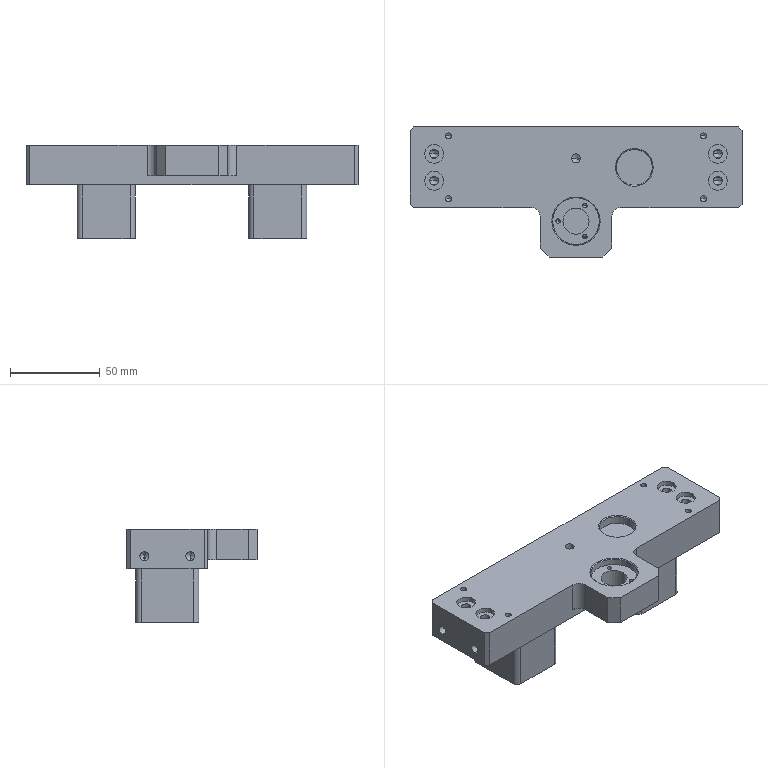NC program | NX | posted with a generic post | part box 185 x 72.5 x 52 mm
Lines 57 to 1270 of 6926:
(CAVITY_MILL , TOOL : D10)
N100 T15 M6
N102 G54
N104 G17 G0 G90 X-4.33 Y48.246 S9500 M3
N106 G43 Z30. H15
N108 Z0.003
N110 G94 G1 Z-0.997 F700.
N112 X-0.866 Y42.246
N114 G3 X0. Y41.746 R1.
N116 G1 X97.503 F2500.
N118 G2 X97.996 Y41.253 R0.493
N120 G1 Y-41.253
N122 G2 X97.503 Y-41.746 R0.493
N124 G1 X-97.503
N126 G2 X-97.996 Y-41.253 R0.493
N128 G1 Y41.253
N130 G2 X-97.503 Y41.746 R0.493
N132 G1 X0.
N134 Y36.746
N136 X92.996
N138 Y-36.746
N140 X64.26
N142 G3 X70.1 Y-28.25 R9.1
N144 G1 Y0.75
N146 G3 X61. Y9.85 R9.1
N148 G1 X34.5
N150 G3 X25.4 Y0.75 R9.1
N152 G1 Y-28.25
N154 G3 X31.24 Y-36.746 R9.1
N156 G1 X31.598 Y-35.812
N158 G2 X26.4 Y-28.25 R8.1
N160 G1 Y0.75
N162 G2 X34.5 Y8.85 R8.1
N164 G1 X61.
N166 G2 X69.1 Y0.75 R8.1
N168 G1 Y-28.25
N170 G2 X61. Y-36.35 R8.1
N172 G1 X34.5
N174 G2 X31.598 Y-35.812 R8.1
N176 G1 X31.24 Y-36.746
N178 X-31.24
N180 G3 X-25.4 Y-28.25 R9.1
N182 G1 Y0.75
N184 G3 X-34.5 Y9.85 R9.1
N186 G1 X-61.
N188 G3 X-70.1 Y0.75 R9.1
N190 G1 Y-28.25
N192 G3 X-64.26 Y-36.746 R9.1
N194 G1 X-63.902 Y-35.812
N196 G2 X-69.1 Y-28.25 R8.1
N198 G1 Y0.75
N200 G2 X-61. Y8.85 R8.1
N202 G1 X-34.5
N204 G2 X-26.4 Y0.75 R8.1
N206 G1 Y-28.25
N208 G2 X-34.5 Y-36.35 R8.1
N210 G1 X-61.
N212 G2 X-63.902 Y-35.812 R8.1
N214 G1 X-64.26 Y-36.746
N216 X-92.996
N218 Y36.746
N220 X0.
N222 Y31.746
N224 X87.996
N226 Y-31.746
N228 X74.66
N230 G3 X75.1 Y-28.25 R14.1
N232 G1 Y0.75
N234 G3 X61. Y14.85 R14.1
N236 G1 X34.5
N238 G3 X20.4 Y0.75 R14.1
N240 G1 Y-28.25
N242 G3 X20.84 Y-31.746 R14.1
N244 G1 X-20.84
N246 G3 X-20.4 Y-28.25 R14.1
N248 G1 Y0.75
N250 G3 X-34.5 Y14.85 R14.1
N252 G1 X-61.
N254 G3 X-75.1 Y0.75 R14.1
N256 G1 Y-28.25
N258 G3 X-74.66 Y-31.746 R14.1
N260 G1 X-87.996
N262 Y31.746
N264 X0.
N266 Y26.746
N268 X82.996
N270 Y-26.746
N272 X80.1
N274 Y0.75
N276 G3 X70.376 Y17.39 R19.1
N278 G1 X72.831 Y21.746
N280 X77.996
N282 Y17.836
N284 G3 X72.831 Y21.746 R24.1
N286 G1 X70.376 Y17.39
N288 G3 X61. Y19.85 R19.1
N290 G1 X34.5
N292 G3 X15.4 Y0.75 R19.1
N294 G1 Y-26.746
N296 X-15.4
N298 Y0.75
N300 G3 X-34.5 Y19.85 R19.1
N302 G1 X-61.
N304 G3 X-80.1 Y0.75 R19.1
N306 G1 Y-26.746
N308 X-82.996
N310 Y26.746
N312 X-72.831
N314 Y21.746
N316 G3 X-77.996 Y17.836 R24.1
N318 G1 Y21.746
N320 X-72.831
N322 Y26.746
N324 X0.
N326 Y21.746
N328 X22.669
N330 G3 X10.4 Y0.75 R24.1
N332 G1 Y-21.746
N334 X-10.4
N336 Y0.75
N338 G3 X-22.669 Y21.746 R24.1
N340 G1 X0.
N342 Y16.746
N344 X10.191
N346 G3 X5.4 Y0.75 R29.1
N348 G1 Y-16.746
N350 X-5.4
N352 Y0.75
N354 G3 X-10.191 Y16.746 R29.1
N356 G1 X0.
N358 Y11.746
N360 X2.222
N362 G3 X0.4 Y0.75 R34.1
N364 G1 Y-11.746
N366 X-0.4
N368 Y0.75
N370 G3 X-2.222 Y11.746 R34.1
N372 G1 X0.
N374 G3 X0.866 Y12.246 R1.
N376 G1 Z0.003
N378 G0 X-4.33 Y48.246 Z-0.993
N380 G1 Z-1.993 F700.
N382 X-0.866 Y42.246
N384 G3 X0. Y41.746 R1.
N386 G1 X97.503 F2500.
N388 G2 X97.996 Y41.253 R0.493
N390 G1 Y-41.253
N392 G2 X97.503 Y-41.746 R0.493
N394 G1 X-97.503
N396 G2 X-97.996 Y-41.253 R0.493
N398 G1 Y41.253
N400 G2 X-97.503 Y41.746 R0.493
N402 G1 X0.
N404 Y36.746
N406 X92.996
N408 Y-36.746
N410 X64.26
N412 G3 X70.1 Y-28.25 R9.1
N414 G1 Y0.75
N416 G3 X61. Y9.85 R9.1
N418 G1 X34.5
N420 G3 X25.4 Y0.75 R9.1
N422 G1 Y-28.25
N424 G3 X31.24 Y-36.746 R9.1
N426 G1 X31.599 Y-35.813
N428 G2 X26.4 Y-28.25 R8.1
N430 G1 Y0.75
N432 G2 X34.5 Y8.85 R8.1
N434 G1 X61.
N436 G2 X69.1 Y0.75 R8.1
N438 G1 Y-28.25
N440 G2 X61. Y-36.35 R8.1
N442 G1 X34.5
N444 G2 X31.599 Y-35.813 R8.1
N446 G1 X31.24 Y-36.746
N448 X-31.24
N450 G3 X-25.4 Y-28.25 R9.1
N452 G1 Y0.75
N454 G3 X-34.5 Y9.85 R9.1
N456 G1 X-61.
N458 G3 X-70.1 Y0.75 R9.1
N460 G1 Y-28.25
N462 G3 X-64.26 Y-36.746 R9.1
N464 G1 X-63.901 Y-35.813
N466 G2 X-69.1 Y-28.25 R8.1
N468 G1 Y0.75
N470 G2 X-61. Y8.85 R8.1
N472 G1 X-34.5
N474 G2 X-26.4 Y0.75 R8.1
N476 G1 Y-28.25
N478 G2 X-34.5 Y-36.35 R8.1
N480 G1 X-61.
N482 G2 X-63.901 Y-35.813 R8.1
N484 G1 X-64.26 Y-36.746
N486 X-92.996
N488 Y36.746
N490 X0.
N492 Y31.746
N494 X87.996
N496 Y-31.746
N498 X74.66
N500 G3 X75.1 Y-28.25 R14.1
N502 G1 Y0.75
N504 G3 X61. Y14.85 R14.1
N506 G1 X34.5
N508 G3 X20.4 Y0.75 R14.1
N510 G1 Y-28.25
N512 G3 X20.84 Y-31.746 R14.1
N514 G1 X-20.84
N516 G3 X-20.4 Y-28.25 R14.1
N518 G1 Y0.75
N520 G3 X-34.5 Y14.85 R14.1
N522 G1 X-61.
N524 G3 X-75.1 Y0.75 R14.1
N526 G1 Y-28.25
N528 G3 X-74.66 Y-31.746 R14.1
N530 G1 X-87.996
N532 Y31.746
N534 X0.
N536 Y26.746
N538 X82.996
N540 Y-26.746
N542 X80.1
N544 Y0.75
N546 G3 X70.376 Y17.39 R19.1
N548 G1 X72.831 Y21.746
N550 X77.996
N552 Y17.836
N554 G3 X72.831 Y21.746 R24.1
N556 G1 X70.376 Y17.39
N558 G3 X61. Y19.85 R19.1
N560 G1 X34.5
N562 G3 X15.4 Y0.75 R19.1
N564 G1 Y-26.746
N566 X-15.4
N568 Y0.75
N570 G3 X-34.5 Y19.85 R19.1
N572 G1 X-61.
N574 G3 X-80.1 Y0.75 R19.1
N576 G1 Y-26.746
N578 X-82.996
N580 Y26.746
N582 X-72.831
N584 Y21.746
N586 G3 X-77.996 Y17.836 R24.1
N588 G1 Y21.746
N590 X-72.831
N592 Y26.746
N594 X0.
N596 Y21.746
N598 X22.669
N600 G3 X10.4 Y0.75 R24.1
N602 G1 Y-21.746
N604 X-10.4
N606 Y0.75
N608 G3 X-22.669 Y21.746 R24.1
N610 G1 X0.
N612 Y16.746
N614 X10.191
N616 G3 X5.4 Y0.75 R29.1
N618 G1 Y-16.746
N620 X-5.4
N622 Y0.75
N624 G3 X-10.191 Y16.746 R29.1
N626 G1 X0.
N628 Y11.746
N630 X2.222
N632 G3 X0.4 Y0.75 R34.1
N634 G1 Y-11.746
N636 X-0.4
N638 Y0.75
N640 G3 X-2.222 Y11.746 R34.1
N642 G1 X0.
N644 G3 X0.866 Y12.246 R1.
N646 G1 Z-0.993
N648 G0 X-4.33 Y48.246 Z-1.99
N650 G1 Z-2.99 F700.
N652 X-0.866 Y42.246
N654 G3 X0. Y41.746 R1.
N656 G1 X97.503 F2500.
N658 G2 X97.997 Y41.253 R0.493
N660 G1 Y-41.253
N662 G2 X97.503 Y-41.746 R0.493
N664 G1 X-97.503
N666 G2 X-97.997 Y-41.253 R0.493
N668 G1 Y41.253
N670 G2 X-97.503 Y41.746 R0.493
N672 G1 X0.
N674 Y36.746
N676 X92.997
N678 Y-36.746
N680 X64.259
N682 G3 X70.1 Y-28.25 R9.1
N684 G1 Y0.75
N686 G3 X61. Y9.85 R9.1
N688 G1 X34.5
N690 G3 X25.4 Y0.75 R9.1
N692 G1 Y-28.25
N694 G3 X31.241 Y-36.746 R9.1
N696 G1 X31.599 Y-35.813
N698 G2 X26.4 Y-28.25 R8.1
N700 G1 Y0.75
N702 G2 X34.5 Y8.85 R8.1
N704 G1 X61.
N706 G2 X69.1 Y0.75 R8.1
N708 G1 Y-28.25
N710 G2 X61. Y-36.35 R8.1
N712 G1 X34.5
N714 G2 X31.599 Y-35.813 R8.1
N716 G1 X31.241 Y-36.746
N718 X-31.241
N720 G3 X-25.4 Y-28.25 R9.1
N722 G1 Y0.75
N724 G3 X-34.5 Y9.85 R9.1
N726 G1 X-61.
N728 G3 X-70.1 Y0.75 R9.1
N730 G1 Y-28.25
N732 G3 X-64.259 Y-36.746 R9.1
N734 G1 X-63.901 Y-35.813
N736 G2 X-69.1 Y-28.25 R8.1
N738 G1 Y0.75
N740 G2 X-61. Y8.85 R8.1
N742 G1 X-34.5
N744 G2 X-26.4 Y0.75 R8.1
N746 G1 Y-28.25
N748 G2 X-34.5 Y-36.35 R8.1
N750 G1 X-61.
N752 G2 X-63.901 Y-35.813 R8.1
N754 G1 X-64.259 Y-36.746
N756 X-92.997
N758 Y36.746
N760 X0.
N762 Y31.746
N764 X87.997
N766 Y-31.746
N768 X74.66
N770 G3 X75.1 Y-28.25 R14.1
N772 G1 Y0.75
N774 G3 X61. Y14.85 R14.1
N776 G1 X34.5
N778 G3 X20.4 Y0.75 R14.1
N780 G1 Y-28.25
N782 G3 X20.84 Y-31.746 R14.1
N784 G1 X-20.84
N786 G3 X-20.4 Y-28.25 R14.1
N788 G1 Y0.75
N790 G3 X-34.5 Y14.85 R14.1
N792 G1 X-61.
N794 G3 X-75.1 Y0.75 R14.1
N796 G1 Y-28.25
N798 G3 X-74.66 Y-31.746 R14.1
N800 G1 X-87.997
N802 Y31.746
N804 X0.
N806 Y26.746
N808 X82.997
N810 Y-26.746
N812 X80.1
N814 Y0.75
N816 G3 X70.376 Y17.39 R19.1
N818 G1 X72.831 Y21.746
N820 X77.997
N822 Y17.836
N824 G3 X72.831 Y21.746 R24.1
N826 G1 X70.376 Y17.39
N828 G3 X61. Y19.85 R19.1
N830 G1 X34.5
N832 G3 X15.4 Y0.75 R19.1
N834 G1 Y-26.746
N836 X-15.4
N838 Y0.75
N840 G3 X-34.5 Y19.85 R19.1
N842 G1 X-61.
N844 G3 X-80.1 Y0.75 R19.1
N846 G1 Y-26.746
N848 X-82.997
N850 Y26.746
N852 X-72.831
N854 Y21.746
N856 G3 X-77.997 Y17.836 R24.1
N858 G1 Y21.746
N860 X-72.831
N862 Y26.746
N864 X0.
N866 Y21.746
N868 X22.669
N870 G3 X10.4 Y0.75 R24.1
N872 G1 Y-21.746
N874 X-10.4
N876 Y0.75
N878 G3 X-22.669 Y21.746 R24.1
N880 G1 X0.
N882 Y16.746
N884 X10.191
N886 G3 X5.4 Y0.75 R29.1
N888 G1 Y-16.746
N890 X-5.4
N892 Y0.75
N894 G3 X-10.191 Y16.746 R29.1
N896 G1 X0.
N898 Y11.746
N900 X2.222
N902 G3 X0.4 Y0.75 R34.1
N904 G1 Y-11.746
N906 X-0.4
N908 Y0.75
N910 G3 X-2.222 Y11.746 R34.1
N912 G1 X0.
N914 G3 X0.866 Y12.246 R1.
N916 G1 Z-1.99
N918 G0 X-4.33 Y48.246 Z-2.987
N920 G1 Z-3.987 F700.
N922 X-0.866 Y42.246
N924 G3 X0. Y41.746 R1.
N926 G1 X97.503 F2500.
N928 G2 X97.997 Y41.253 R0.494
N930 G1 Y-41.253
N932 G2 X97.503 Y-41.746 R0.494
N934 G1 X-97.503
N936 G2 X-97.997 Y-41.253 R0.494
N938 G1 Y41.253
N940 G2 X-97.503 Y41.746 R0.494
N942 G1 X0.
N944 Y36.746
N946 X92.997
N948 Y-36.746
N950 X64.259
N952 G3 X70.1 Y-28.25 R9.1
N954 G1 Y0.75
N956 G3 X61. Y9.85 R9.1
N958 G1 X34.5
N960 G3 X25.4 Y0.75 R9.1
N962 G1 Y-28.25
N964 G3 X31.241 Y-36.746 R9.1
N966 G1 X31.599 Y-35.813
N968 G2 X26.4 Y-28.25 R8.1
N970 G1 Y0.75
N972 G2 X34.5 Y8.85 R8.1
N974 G1 X61.
N976 G2 X69.1 Y0.75 R8.1
N978 G1 Y-28.25
N980 G2 X61. Y-36.35 R8.1
N982 G1 X34.5
N984 G2 X31.599 Y-35.813 R8.1
N986 G1 X31.241 Y-36.746
N988 X-31.241
N990 G3 X-25.4 Y-28.25 R9.1
N992 G1 Y0.75
N994 G3 X-34.5 Y9.85 R9.1
N996 G1 X-61.
N998 G3 X-70.1 Y0.75 R9.1
N1000 G1 Y-28.25
N1002 G3 X-64.259 Y-36.746 R9.1
N1004 G1 X-63.901 Y-35.813
N1006 G2 X-69.1 Y-28.25 R8.1
N1008 G1 Y0.75
N1010 G2 X-61. Y8.85 R8.1
N1012 G1 X-34.5
N1014 G2 X-26.4 Y0.75 R8.1
N1016 G1 Y-28.25
N1018 G2 X-34.5 Y-36.35 R8.1
N1020 G1 X-61.
N1022 G2 X-63.901 Y-35.813 R8.1
N1024 G1 X-64.259 Y-36.746
N1026 X-92.997
N1028 Y36.746
N1030 X0.
N1032 Y31.746
N1034 X87.997
N1036 Y-31.746
N1038 X74.66
N1040 G3 X75.1 Y-28.25 R14.1
N1042 G1 Y0.75
N1044 G3 X61. Y14.85 R14.1
N1046 G1 X34.5
N1048 G3 X20.4 Y0.75 R14.1
N1050 G1 Y-28.25
N1052 G3 X20.84 Y-31.746 R14.1
N1054 G1 X-20.84
N1056 G3 X-20.4 Y-28.25 R14.1
N1058 G1 Y0.75
N1060 G3 X-34.5 Y14.85 R14.1
N1062 G1 X-61.
N1064 G3 X-75.1 Y0.75 R14.1
N1066 G1 Y-28.25
N1068 G3 X-74.66 Y-31.746 R14.1
N1070 G1 X-87.997
N1072 Y31.746
N1074 X0.
N1076 Y26.746
N1078 X82.997
N1080 Y-26.746
N1082 X80.1
N1084 Y0.75
N1086 G3 X70.376 Y17.39 R19.1
N1088 G1 X72.831 Y21.746
N1090 X77.997
N1092 Y17.836
N1094 G3 X72.831 Y21.746 R24.1
N1096 G1 X70.376 Y17.39
N1098 G3 X61. Y19.85 R19.1
N1100 G1 X34.5
N1102 G3 X15.4 Y0.75 R19.1
N1104 G1 Y-26.746
N1106 X-15.4
N1108 Y0.75
N1110 G3 X-34.5 Y19.85 R19.1
N1112 G1 X-61.
N1114 G3 X-80.1 Y0.75 R19.1
N1116 G1 Y-26.746
N1118 X-82.997
N1120 Y26.746
N1122 X-72.831
N1124 Y21.746
N1126 G3 X-77.997 Y17.836 R24.1
N1128 G1 Y21.746
N1130 X-72.831
N1132 Y26.746
N1134 X0.
N1136 Y21.746
N1138 X22.669
N1140 G3 X10.4 Y0.75 R24.1
N1142 G1 Y-21.746
N1144 X-10.4
N1146 Y0.75
N1148 G3 X-22.669 Y21.746 R24.1
N1150 G1 X0.
N1152 Y16.746
N1154 X10.191
N1156 G3 X5.4 Y0.75 R29.1
N1158 G1 Y-16.746
N1160 X-5.4
N1162 Y0.75
N1164 G3 X-10.191 Y16.746 R29.1
N1166 G1 X0.
N1168 Y11.746
N1170 X2.222
N1172 G3 X0.4 Y0.75 R34.1
N1174 G1 Y-11.746
N1176 X-0.4
N1178 Y0.75
N1180 G3 X-2.222 Y11.746 R34.1
N1182 G1 X0.
N1184 G3 X0.866 Y12.246 R1.
N1186 G1 Z-2.987
N1188 G0 X-4.33 Y48.246 Z-3.983
N1190 G1 Z-4.983 F700.
N1192 X-0.866 Y42.246
N1194 G3 X0. Y41.746 R1.
N1196 G1 X97.503 F2500.
N1198 G2 X97.997 Y41.253 R0.494
N1200 G1 Y-41.253
N1202 G2 X97.503 Y-41.746 R0.494
N1204 G1 X-97.503
N1206 G2 X-97.997 Y-41.253 R0.494
N1208 G1 Y41.253
N1210 G2 X-97.503 Y41.746 R0.494
N1212 G1 X0.
N1214 Y36.746
N1216 X92.997
N1218 Y-36.746
N1220 X64.259
N1222 G3 X70.1 Y-28.25 R9.1
N1224 G1 Y0.75
N1226 G3 X61. Y9.85 R9.1
N1228 G1 X34.5
N1230 G3 X25.4 Y0.75 R9.1
N1232 G1 Y-28.25
N1234 G3 X31.241 Y-36.746 R9.1
N1236 G1 X31.599 Y-35.813
N1238 G2 X26.4 Y-28.25 R8.1
N1240 G1 Y0.75
N1242 G2 X34.5 Y8.85 R8.1
N1244 G1 X61.
N1246 G2 X69.1 Y0.75 R8.1
N1248 G1 Y-28.25
N1250 G2 X61. Y-36.35 R8.1
N1252 G1 X34.5
N1254 G2 X31.599 Y-35.813 R8.1
N1256 G1 X31.241 Y-36.746
N1258 X-31.241
N1260 G3 X-25.4 Y-28.25 R9.1
N1262 G1 Y0.75
N1264 G3 X-34.5 Y9.85 R9.1
N1266 G1 X-61.
N1268 G3 X-70.1 Y0.75 R9.1
N1270 G1 Y-28.25
N1272 G3 X-64.259 Y-36.746 R9.1
N1274 G1 X-63.901 Y-35.813
N1276 G2 X-69.1 Y-28.25 R8.1
N1278 G1 Y0.75
N1280 G2 X-61. Y8.85 R8.1
N1282 G1 X-34.5
N1284 G2 X-26.4 Y0.75 R8.1
N1286 G1 Y-28.25
N1288 G2 X-34.5 Y-36.35 R8.1
N1290 G1 X-61.
N1292 G2 X-63.901 Y-35.813 R8.1
N1294 G1 X-64.259 Y-36.746
N1296 X-92.997
N1298 Y36.746
N1300 X0.
N1302 Y31.746
N1304 X87.997
N1306 Y-31.746
N1308 X74.66
N1310 G3 X75.1 Y-28.25 R14.1
N1312 G1 Y0.75
N1314 G3 X61. Y14.85 R14.1
N1316 G1 X34.5
N1318 G3 X20.4 Y0.75 R14.1
N1320 G1 Y-28.25
N1322 G3 X20.84 Y-31.746 R14.1
N1324 G1 X-20.84
N1326 G3 X-20.4 Y-28.25 R14.1
N1328 G1 Y0.75
N1330 G3 X-34.5 Y14.85 R14.1
N1332 G1 X-61.
N1334 G3 X-75.1 Y0.75 R14.1
N1336 G1 Y-28.25
N1338 G3 X-74.66 Y-31.746 R14.1
N1340 G1 X-87.997
N1342 Y31.746
N1344 X0.
N1346 Y26.746
N1348 X82.997
N1350 Y-26.746
N1352 X80.1
N1354 Y0.75
N1356 G3 X70.376 Y17.39 R19.1
N1358 G1 X72.831 Y21.746
N1360 X77.997
N1362 Y17.836
N1364 G3 X72.831 Y21.746 R24.1
N1366 G1 X70.376 Y17.39
N1368 G3 X61. Y19.85 R19.1
N1370 G1 X34.5
N1372 G3 X15.4 Y0.75 R19.1
N1374 G1 Y-26.746
N1376 X-15.4
N1378 Y0.75
N1380 G3 X-34.5 Y19.85 R19.1
N1382 G1 X-61.
N1384 G3 X-80.1 Y0.75 R19.1
N1386 G1 Y-26.746
N1388 X-82.997
N1390 Y26.746
N1392 X-72.831
N1394 Y21.746
N1396 G3 X-77.997 Y17.836 R24.1
N1398 G1 Y21.746
N1400 X-72.831
N1402 Y26.746
N1404 X0.
N1406 Y21.746
N1408 X22.669
N1410 G3 X10.4 Y0.75 R24.1
N1412 G1 Y-21.746
N1414 X-10.4
N1416 Y0.75
N1418 G3 X-22.669 Y21.746 R24.1
N1420 G1 X0.
N1422 Y16.746
N1424 X10.191
N1426 G3 X5.4 Y0.75 R29.1
N1428 G1 Y-16.746
N1430 X-5.4
N1432 Y0.75
N1434 G3 X-10.191 Y16.746 R29.1
N1436 G1 X0.
N1438 Y11.746
N1440 X2.222
N1442 G3 X0.4 Y0.75 R34.1
N1444 G1 Y-11.746
N1446 X-0.4
N1448 Y0.75
N1450 G3 X-2.222 Y11.746 R34.1
N1452 G1 X0.
N1454 G3 X0.866 Y12.246 R1.
N1456 G1 Z-3.983
N1458 G0 X-4.33 Y48.246 Z-4.98
N1460 G1 Z-5.98 F700.
N1462 X-0.866 Y42.246
N1464 G3 X0. Y41.746 R1.
N1466 G1 X97.503 F2500.
N1468 G2 X97.997 Y41.253 R0.494
N1470 G1 Y-41.253
N1472 G2 X97.503 Y-41.746 R0.494
N1474 G1 X-97.503
N1476 G2 X-97.997 Y-41.253 R0.494
N1478 G1 Y41.253
N1480 G2 X-97.503 Y41.746 R0.494
N1482 G1 X0.
N1484 Y36.746
N1486 X92.997
N1488 Y-36.746
N1490 X64.259
N1492 G3 X70.1 Y-28.25 R9.1
N1494 G1 Y0.75
N1496 G3 X61. Y9.85 R9.1
N1498 G1 X34.5
N1500 G3 X25.4 Y0.75 R9.1
N1502 G1 Y-28.25
N1504 G3 X31.241 Y-36.746 R9.1
N1506 G1 X31.599 Y-35.813
N1508 G2 X26.4 Y-28.25 R8.1
N1510 G1 Y0.75
N1512 G2 X34.5 Y8.85 R8.1
N1514 G1 X61.
N1516 G2 X69.1 Y0.75 R8.1
N1518 G1 Y-28.25
N1520 G2 X61. Y-36.35 R8.1
N1522 G1 X34.5
N1524 G2 X31.599 Y-35.813 R8.1
N1526 G1 X31.241 Y-36.746
N1528 X-31.241
N1530 G3 X-25.4 Y-28.25 R9.1
N1532 G1 Y0.75
N1534 G3 X-34.5 Y9.85 R9.1
N1536 G1 X-61.
N1538 G3 X-70.1 Y0.75 R9.1
N1540 G1 Y-28.25
N1542 G3 X-64.259 Y-36.746 R9.1
N1544 G1 X-63.901 Y-35.813
N1546 G2 X-69.1 Y-28.25 R8.1
N1548 G1 Y0.75
N1550 G2 X-61. Y8.85 R8.1
N1552 G1 X-34.5
N1554 G2 X-26.4 Y0.75 R8.1
N1556 G1 Y-28.25
N1558 G2 X-34.5 Y-36.35 R8.1
N1560 G1 X-61.
N1562 G2 X-63.901 Y-35.813 R8.1
N1564 G1 X-64.259 Y-36.746
N1566 X-92.997
N1568 Y36.746
N1570 X0.
N1572 Y31.746
N1574 X87.997
N1576 Y-31.746
N1578 X74.66
N1580 G3 X75.1 Y-28.25 R14.1
N1582 G1 Y0.75
N1584 G3 X61. Y14.85 R14.1
N1586 G1 X34.5
N1588 G3 X20.4 Y0.75 R14.1
N1590 G1 Y-28.25
N1592 G3 X20.84 Y-31.746 R14.1
N1594 G1 X-20.84
N1596 G3 X-20.4 Y-28.25 R14.1
N1598 G1 Y0.75
N1600 G3 X-34.5 Y14.85 R14.1
N1602 G1 X-61.
N1604 G3 X-75.1 Y0.75 R14.1
N1606 G1 Y-28.25
N1608 G3 X-74.66 Y-31.746 R14.1
N1610 G1 X-87.997
N1612 Y31.746
N1614 X0.
N1616 Y26.746
N1618 X82.997
N1620 Y-26.746
N1622 X80.1
N1624 Y0.75
N1626 G3 X70.376 Y17.39 R19.1
N1628 G1 X72.83 Y21.746
N1630 X77.997
N1632 Y17.836
N1634 G3 X72.83 Y21.746 R24.1
N1636 G1 X70.376 Y17.39
N1638 G3 X61. Y19.85 R19.1
N1640 G1 X34.5
N1642 G3 X15.4 Y0.75 R19.1
N1644 G1 Y-26.746
N1646 X-15.4
N1648 Y0.75
N1650 G3 X-34.5 Y19.85 R19.1
N1652 G1 X-61.
N1654 G3 X-80.1 Y0.75 R19.1
N1656 G1 Y-26.746
N1658 X-82.997
N1660 Y26.746
N1662 X-72.83
N1664 Y21.746
N1666 G3 X-77.997 Y17.836 R24.1
N1668 G1 Y21.746
N1670 X-72.83
N1672 Y26.746
N1674 X0.
N1676 Y21.746
N1678 X22.67
N1680 G3 X10.4 Y0.75 R24.1
N1682 G1 Y-21.746
N1684 X-10.4
N1686 Y0.75
N1688 G3 X-22.67 Y21.746 R24.1
N1690 G1 X0.
N1692 Y16.746
N1694 X10.191
N1696 G3 X5.4 Y0.75 R29.1
N1698 G1 Y-16.746
N1700 X-5.4
N1702 Y0.75
N1704 G3 X-10.191 Y16.746 R29.1
N1706 G1 X0.
N1708 Y11.746
N1710 X2.222
N1712 G3 X0.4 Y0.75 R34.1
N1714 G1 Y-11.746
N1716 X-0.4
N1718 Y0.75
N1720 G3 X-2.222 Y11.746 R34.1
N1722 G1 X0.
N1724 G3 X0.866 Y12.246 R1.
N1726 G1 Z-4.98
N1728 G0 X-4.33 Y48.247 Z-5.977
N1730 G1 Z-6.977 F700.
N1732 X-0.866 Y42.247
N1734 G3 X0. Y41.747 R1.
N1736 G1 X97.503 F2500.
N1738 G2 X97.997 Y41.253 R0.494
N1740 G1 Y-41.253
N1742 G2 X97.503 Y-41.747 R0.494
N1744 G1 X-97.503
N1746 G2 X-97.997 Y-41.253 R0.494
N1748 G1 Y41.253
N1750 G2 X-97.503 Y41.747 R0.494
N1752 G1 X0.
N1754 Y36.747
N1756 X92.997
N1758 Y-36.747
N1760 X64.259
N1762 G3 X70.1 Y-28.25 R9.1
N1764 G1 Y0.75
N1766 G3 X61. Y9.85 R9.1
N1768 G1 X34.5
N1770 G3 X25.4 Y0.75 R9.1
N1772 G1 Y-28.25
N1774 G3 X31.241 Y-36.747 R9.1
N1776 G1 X31.599 Y-35.813
N1778 G2 X26.4 Y-28.25 R8.1
N1780 G1 Y0.75
N1782 G2 X34.5 Y8.85 R8.1
N1784 G1 X61.
N1786 G2 X69.1 Y0.75 R8.1
N1788 G1 Y-28.25
N1790 G2 X61. Y-36.35 R8.1
N1792 G1 X34.5
N1794 G2 X31.599 Y-35.813 R8.1
N1796 G1 X31.241 Y-36.747
N1798 X-31.241
N1800 G3 X-25.4 Y-28.25 R9.1
N1802 G1 Y0.75
N1804 G3 X-34.5 Y9.85 R9.1
N1806 G1 X-61.
N1808 G3 X-70.1 Y0.75 R9.1
N1810 G1 Y-28.25
N1812 G3 X-64.259 Y-36.747 R9.1
N1814 G1 X-63.901 Y-35.813
N1816 G2 X-69.1 Y-28.25 R8.1
N1818 G1 Y0.75
N1820 G2 X-61. Y8.85 R8.1
N1822 G1 X-34.5
N1824 G2 X-26.4 Y0.75 R8.1
N1826 G1 Y-28.25
N1828 G2 X-34.5 Y-36.35 R8.1
N1830 G1 X-61.
N1832 G2 X-63.901 Y-35.813 R8.1
N1834 G1 X-64.259 Y-36.747
N1836 X-92.997
N1838 Y36.747
N1840 X0.
N1842 Y31.747
N1844 X87.997
N1846 Y-31.747
N1848 X74.66
N1850 G3 X75.1 Y-28.25 R14.1
N1852 G1 Y0.75
N1854 G3 X61. Y14.85 R14.1
N1856 G1 X34.5
N1858 G3 X20.4 Y0.75 R14.1
N1860 G1 Y-28.25
N1862 G3 X20.84 Y-31.747 R14.1
N1864 G1 X-20.84
N1866 G3 X-20.4 Y-28.25 R14.1
N1868 G1 Y0.75
N1870 G3 X-34.5 Y14.85 R14.1
N1872 G1 X-61.
N1874 G3 X-75.1 Y0.75 R14.1
N1876 G1 Y-28.25
N1878 G3 X-74.66 Y-31.747 R14.1
N1880 G1 X-87.997
N1882 Y31.747
N1884 X0.
N1886 Y26.747
N1888 X82.997
N1890 Y-26.747
N1892 X80.1
N1894 Y0.75
N1896 G3 X70.376 Y17.39 R19.1
N1898 G1 X72.83 Y21.747
N1900 X77.997
N1902 Y17.836
N1904 G3 X72.83 Y21.747 R24.1
N1906 G1 X70.376 Y17.39
N1908 G3 X61. Y19.85 R19.1
N1910 G1 X34.5
N1912 G3 X15.4 Y0.75 R19.1
N1914 G1 Y-26.747
N1916 X-15.4
N1918 Y0.75
N1920 G3 X-34.5 Y19.85 R19.1
N1922 G1 X-61.
N1924 G3 X-80.1 Y0.75 R19.1
N1926 G1 Y-26.747
N1928 X-82.997
N1930 Y26.747
N1932 X-72.83
N1934 Y21.747
N1936 G3 X-77.997 Y17.836 R24.1
N1938 G1 Y21.747
N1940 X-72.83
N1942 Y26.747
N1944 X0.
N1946 Y21.747
N1948 X22.67
N1950 G3 X10.4 Y0.75 R24.1
N1952 G1 Y-21.747
N1954 X-10.4
N1956 Y0.75
N1958 G3 X-22.67 Y21.747 R24.1
N1960 G1 X0.
N1962 Y16.747
N1964 X10.191
N1966 G3 X5.4 Y0.75 R29.1
N1968 G1 Y-16.747
N1970 X-5.4
N1972 Y0.75
N1974 G3 X-10.191 Y16.747 R29.1
N1976 G1 X0.
N1978 Y11.747
N1980 X2.222
N1982 G3 X0.4 Y0.75 R34.1
N1984 G1 Y-11.747
N1986 X-0.4
N1988 Y0.75
N1990 G3 X-2.222 Y11.747 R34.1
N1992 G1 X0.
N1994 G3 X0.866 Y12.247 R1.
N1996 G1 Z-5.977
N1998 G0 X-4.33 Y48.247 Z-6.973
N2000 G1 Z-7.973 F700.
N2002 X-0.866 Y42.247
N2004 G3 X0. Y41.747 R1.
N2006 G1 X97.503 F2500.
N2008 G2 X97.997 Y41.253 R0.494
N2010 G1 Y-41.253
N2012 G2 X97.503 Y-41.747 R0.494
N2014 G1 X-97.503
N2016 G2 X-97.997 Y-41.253 R0.494
N2018 G1 Y41.253
N2020 G2 X-97.503 Y41.747 R0.494
N2022 G1 X0.
N2024 Y36.747
N2026 X92.997
N2028 Y-36.747
N2030 X64.258
N2032 G3 X70.1 Y-28.25 R9.1
N2034 G1 Y0.75
N2036 G3 X61. Y9.85 R9.1
N2038 G1 X34.5
N2040 G3 X25.4 Y0.75 R9.1
N2042 G1 Y-28.25
N2044 G3 X31.242 Y-36.747 R9.1
N2046 G1 X31.6 Y-35.813
N2048 G2 X26.4 Y-28.25 R8.1
N2050 G1 Y0.75
N2052 G2 X34.5 Y8.85 R8.1
N2054 G1 X61.
N2056 G2 X69.1 Y0.75 R8.1
N2058 G1 Y-28.25
N2060 G2 X61. Y-36.35 R8.1
N2062 G1 X34.5
N2064 G2 X31.6 Y-35.813 R8.1
N2066 G1 X31.242 Y-36.747
N2068 X-31.242
N2070 G3 X-25.4 Y-28.25 R9.1
N2072 G1 Y0.75
N2074 G3 X-34.5 Y9.85 R9.1
N2076 G1 X-61.
N2078 G3 X-70.1 Y0.75 R9.1
N2080 G1 Y-28.25
N2082 G3 X-64.258 Y-36.747 R9.1
N2084 G1 X-63.9 Y-35.813
N2086 G2 X-69.1 Y-28.25 R8.1
N2088 G1 Y0.75
N2090 G2 X-61. Y8.85 R8.1
N2092 G1 X-34.5
N2094 G2 X-26.4 Y0.75 R8.1
N2096 G1 Y-28.25
N2098 G2 X-34.5 Y-36.35 R8.1
N2100 G1 X-61.
N2102 G2 X-63.9 Y-35.813 R8.1
N2104 G1 X-64.258 Y-36.747
N2106 X-92.997
N2108 Y36.747
N2110 X0.
N2112 Y31.747
N2114 X87.997
N2116 Y-31.747
N2118 X74.66
N2120 G3 X75.1 Y-28.25 R14.1
N2122 G1 Y0.75
N2124 G3 X61. Y14.85 R14.1
N2126 G1 X34.5
N2128 G3 X20.4 Y0.75 R14.1
N2130 G1 Y-28.25
N2132 G3 X20.84 Y-31.747 R14.1
N2134 G1 X-20.84
N2136 G3 X-20.4 Y-28.25 R14.1
N2138 G1 Y0.75
N2140 G3 X-34.5 Y14.85 R14.1
N2142 G1 X-61.
N2144 G3 X-75.1 Y0.75 R14.1
N2146 G1 Y-28.25
N2148 G3 X-74.66 Y-31.747 R14.1
N2150 G1 X-87.997
N2152 Y31.747
N2154 X0.
N2156 Y26.747
N2158 X82.997
N2160 Y-26.747
N2162 X80.1
N2164 Y0.75
N2166 G3 X70.376 Y17.39 R19.1
N2168 G1 X72.83 Y21.747
N2170 X77.997
N2172 Y17.836
N2174 G3 X72.83 Y21.747 R24.1
N2176 G1 X70.376 Y17.39
N2178 G3 X61. Y19.85 R19.1
N2180 G1 X34.5
N2182 G3 X15.4 Y0.75 R19.1
N2184 G1 Y-26.747
N2186 X-15.4
N2188 Y0.75
N2190 G3 X-34.5 Y19.85 R19.1
N2192 G1 X-61.
N2194 G3 X-80.1 Y0.75 R19.1
N2196 G1 Y-26.747
N2198 X-82.997
N2200 Y26.747
N2202 X-72.83
N2204 Y21.747
N2206 G3 X-77.997 Y17.836 R24.1
N2208 G1 Y21.747
N2210 X-72.83
N2212 Y26.747
N2214 X0.
N2216 Y21.747
N2218 X22.67
N2220 G3 X10.4 Y0.75 R24.1
N2222 G1 Y-21.747
N2224 X-10.4
N2226 Y0.75
N2228 G3 X-22.67 Y21.747 R24.1
N2230 G1 X0.
N2232 Y16.747
N2234 X10.191
N2236 G3 X5.4 Y0.75 R29.1
N2238 G1 Y-16.747
N2240 X-5.4
N2242 Y0.75
N2244 G3 X-10.191 Y16.747 R29.1
N2246 G1 X0.
N2248 Y11.747
N2250 X2.222
N2252 G3 X0.4 Y0.75 R34.1
N2254 G1 Y-11.747
N2256 X-0.4
N2258 Y0.75
N2260 G3 X-2.222 Y11.747 R34.1
N2262 G1 X0.
N2264 G3 X0.866 Y12.247 R1.
N2266 G1 Z-6.973
N2268 G0 X-4.33 Y48.247 Z-7.97
N2270 G1 Z-8.97 F700.
N2272 X-0.866 Y42.247
N2274 G3 X0. Y41.747 R1.
N2276 G1 X97.503 F2500.
N2278 G2 X97.997 Y41.253 R0.494
N2280 G1 Y-41.253
N2282 G2 X97.503 Y-41.747 R0.494
N2284 G1 X-97.503
N2286 G2 X-97.997 Y-41.253 R0.494
N2288 G1 Y41.253
N2290 G2 X-97.503 Y41.747 R0.494
N2292 G1 X0.
N2294 Y36.747
N2296 X92.997
N2298 Y-36.747
N2300 X64.258
N2302 G3 X70.1 Y-28.25 R9.1
N2304 G1 Y0.75
N2306 G3 X61. Y9.85 R9.1
N2308 G1 X34.5
N2310 G3 X25.4 Y0.75 R9.1
N2312 G1 Y-28.25
N2314 G3 X31.242 Y-36.747 R9.1
N2316 G1 X31.6 Y-35.813
N2318 G2 X26.4 Y-28.25 R8.1
N2320 G1 Y0.75
N2322 G2 X34.5 Y8.85 R8.1
N2324 G1 X61.
N2326 G2 X69.1 Y0.75 R8.1
N2328 G1 Y-28.25
N2330 G2 X61. Y-36.35 R8.1
N2332 G1 X34.5
N2334 G2 X31.6 Y-35.813 R8.1
N2336 G1 X31.242 Y-36.747
N2338 X-31.242
N2340 G3 X-25.4 Y-28.25 R9.1
N2342 G1 Y0.75
N2344 G3 X-34.5 Y9.85 R9.1
N2346 G1 X-61.
N2348 G3 X-70.1 Y0.75 R9.1
N2350 G1 Y-28.25
N2352 G3 X-64.258 Y-36.747 R9.1
N2354 G1 X-63.9 Y-35.813
N2356 G2 X-69.1 Y-28.25 R8.1
N2358 G1 Y0.75
N2360 G2 X-61. Y8.85 R8.1
N2362 G1 X-34.5
N2364 G2 X-26.4 Y0.75 R8.1
N2366 G1 Y-28.25
N2368 G2 X-34.5 Y-36.35 R8.1
N2370 G1 X-61.
N2372 G2 X-63.9 Y-35.813 R8.1
N2374 G1 X-64.258 Y-36.747
N2376 X-92.997
N2378 Y36.747
N2380 X0.
N2382 Y31.747
N2384 X87.997
N2386 Y-31.747
N2388 X74.66
N2390 G3 X75.1 Y-28.25 R14.1
N2392 G1 Y0.75
N2394 G3 X61. Y14.85 R14.1
N2396 G1 X34.5
N2398 G3 X20.4 Y0.75 R14.1
N2400 G1 Y-28.25
N2402 G3 X20.84 Y-31.747 R14.1
N2404 G1 X-20.84
N2406 G3 X-20.4 Y-28.25 R14.1
N2408 G1 Y0.75
N2410 G3 X-34.5 Y14.85 R14.1
N2412 G1 X-61.
N2414 G3 X-75.1 Y0.75 R14.1
N2416 G1 Y-28.25
N2418 G3 X-74.66 Y-31.747 R14.1
N2420 G1 X-87.997
N2422 Y31.747
N2424 X0.
N2426 Y26.747
N2428 X82.997
N2430 Y-26.747
N2432 X80.1
N2434 Y0.75
N2436 G3 X70.376 Y17.391 R19.1
N2438 G1 X72.83 Y21.747
N2440 X77.997
N2442 Y17.835
N2444 G3 X72.83 Y21.747 R24.1
N2446 G1 X70.376 Y17.391
N2448 G3 X61. Y19.85 R19.1
N2450 G1 X34.5
N2452 G3 X15.4 Y0.75 R19.1
N2454 G1 Y-26.747
N2456 X-15.4
N2458 Y0.75
N2460 G3 X-34.5 Y19.85 R19.1
N2462 G1 X-61.
N2464 G3 X-80.1 Y0.75 R19.1
N2466 G1 Y-26.747
N2468 X-82.997
N2470 Y26.747
N2472 X-72.83
N2474 Y21.747
N2476 G3 X-77.997 Y17.835 R24.1
N2478 G1 Y21.747
N2480 X-72.83
N2482 Y26.747
N2484 X0.
N2486 Y21.747
N2488 X22.67
N2490 G3 X10.4 Y0.75 R24.1
N2492 G1 Y-21.747
N2494 X-10.4
N2496 Y0.75
N2498 G3 X-22.67 Y21.747 R24.1
N2500 G1 X0.
N2502 Y16.747
N2504 X10.191
N2506 G3 X5.4 Y0.75 R29.1
N2508 G1 Y-16.747
N2510 X-5.4
N2512 Y0.75
N2514 G3 X-10.191 Y16.747 R29.1
N2516 G1 X0.
N2518 Y11.747
N2520 X2.222